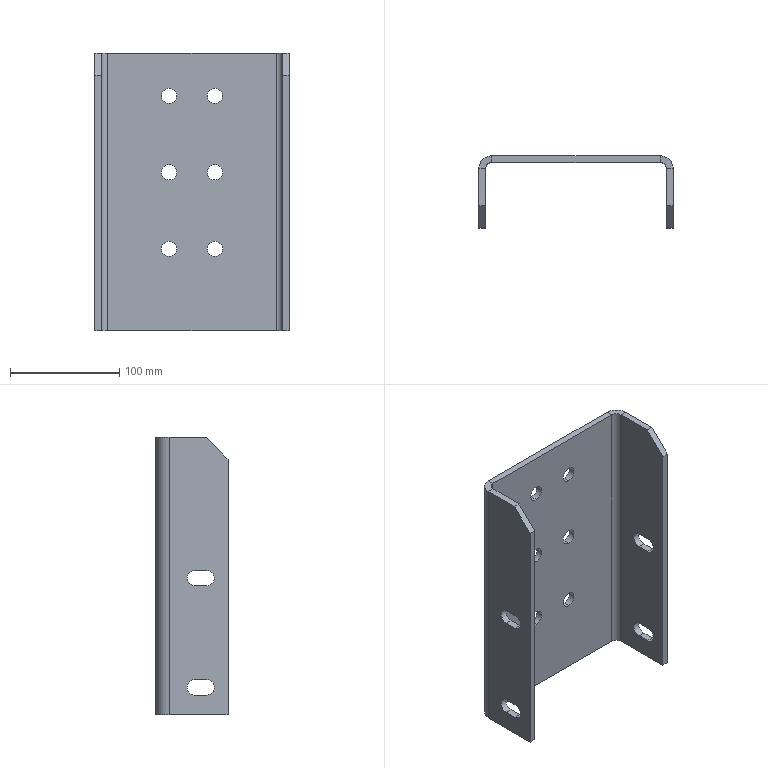Part | STEP file | 02-Driven chain anti-jump bracket 2 | 1 solid | 52 faces | box 178 x 66 x 254 mm | volume 427046 mm3 | plane 28 | cylinder 24 | commonest cylinder face diameters 14 x20 12 x2 24 x2